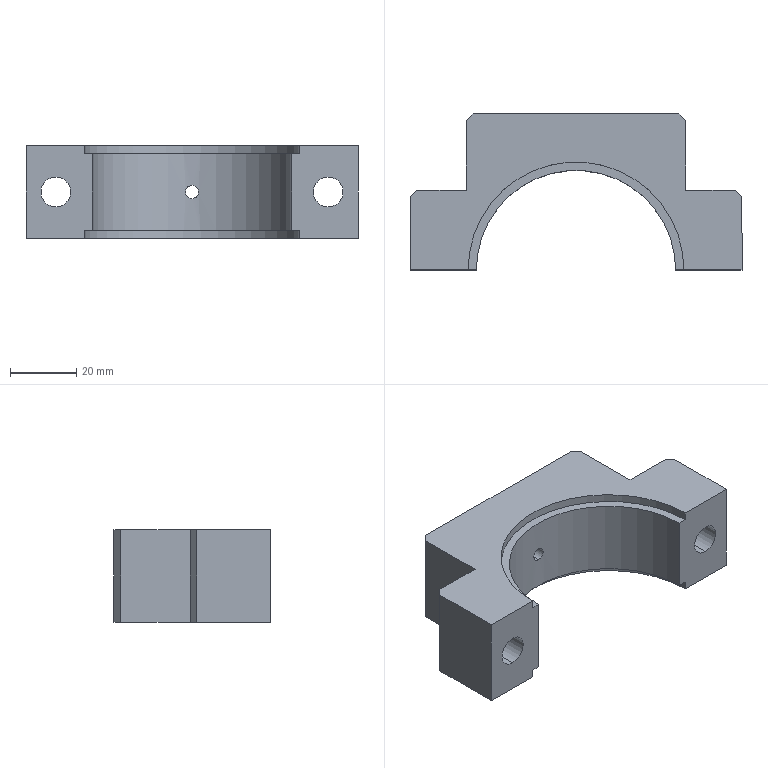Part | SolidWorks | features HoleWzd 3, ICE 2, Chamfer 1, Extrusion 1 | 1 solid | 30 faces | box 100 x 47 x 28 mm | volume 65054 mm3 | plane 17 | cylinder 11 | cone 2 | commonest cylinder face diameters 9 x4 4 x2 7 x2 65 x2 60 x1
STEP:
#1=CARTESIAN_POINT('',(0.,30.,12.));
#2=VERTEX_POINT('',#1);
#3=CARTESIAN_POINT('',(0.,30.,16.));
#4=VERTEX_POINT('',#3);
#5=CARTESIAN_POINT('',(0.,30.,12.));
#6=CARTESIAN_POINT('',(-0.261,30.,12.));
#7=CARTESIAN_POINT('',(-0.5242,29.996,12.052));
#8=CARTESIAN_POINT('',(-1.006,29.984,12.252));
#9=CARTESIAN_POINT('',(-1.229,29.975,12.401));
#10=CARTESIAN_POINT('',(-1.505,29.962,12.677));
#11=CARTESIAN_POINT('',(-1.59,29.958,12.78));
#12=CARTESIAN_POINT('',(-1.735,29.95,12.997));
#13=CARTESIAN_POINT('',(-1.797,29.946,13.112));
#14=CARTESIAN_POINT('',(-1.897,29.94,13.354));
#15=CARTESIAN_POINT('',(-1.936,29.937,13.481));
#16=CARTESIAN_POINT('',(-1.987,29.934,13.737));
#17=CARTESIAN_POINT('',(-2.,29.933,13.866));
#18=CARTESIAN_POINT('',(-2.,29.933,14.13));
#19=CARTESIAN_POINT('',(-1.987,29.934,14.261));
#20=CARTESIAN_POINT('',(-1.937,29.937,14.516));
#21=CARTESIAN_POINT('',(-1.898,29.94,14.643));
#22=CARTESIAN_POINT('',(-1.798,29.946,14.886));
#23=CARTESIAN_POINT('',(-1.737,29.95,15.001));
#24=CARTESIAN_POINT('',(-1.592,29.958,15.218));
#25=CARTESIAN_POINT('',(-1.507,29.962,15.321));
#26=CARTESIAN_POINT('',(-1.323,29.971,15.506));
#27=CARTESIAN_POINT('',(-1.222,29.975,15.588));
#28=CARTESIAN_POINT('',(-1.004,29.983,15.735));
#29=CARTESIAN_POINT('',(-0.8877,29.987,15.797));
#30=CARTESIAN_POINT('',(-0.5269,29.996,15.947));
#31=CARTESIAN_POINT('',(-0.2643,30.,16.));
#32=CARTESIAN_POINT('',(0.,30.,16.));
#33=B_SPLINE_CURVE_WITH_KNOTS('',3,(#5,#6,#7,#8,#9,#10,#11,#12,#13,#14,#15,#16,#17,#18,#19,#20,#21,#22,#23,#24,#25,#26,#27,#28,#29,#30,#31,#32),.UNSPECIFIED.,.F.,.F.,(4,2,2,2,2,2,2,2,2,2,2,2,2,4),(0.006255,0.007036,0.007818,0.008209,0.0086,0.00899,0.009381,0.009772,0.01016,0.01055,0.01094,0.01134,0.01173,0.01251),.UNSPECIFIED.);
#34=EDGE_CURVE('',#2,#4,#33,.T.);
#35=ORIENTED_EDGE('',*,*,#34,.F.);
#36=CARTESIAN_POINT('',(0.,33.099,12.));
#37=VERTEX_POINT('',#36);
#38=CARTESIAN_POINT('',(0.,47.,12.));
#39=DIRECTION('',(0.,1.,0.));
#40=VECTOR('',#39,1000.);
#41=LINE('',#38,#40);
#42=EDGE_CURVE('',#2,#37,#41,.T.);
#43=ORIENTED_EDGE('',*,*,#42,.T.);
#44=CARTESIAN_POINT('',(0.,33.099,16.));
#45=VERTEX_POINT('',#44);
#46=CARTESIAN_POINT('',(0.,33.099,14.));
#47=DIRECTION('',(0.,-1.,0.));
#48=DIRECTION('',(0.,0.,1.));
#49=AXIS2_PLACEMENT_3D('',#46,#47,#48);
#50=CIRCLE('',#49,2.);
#51=EDGE_CURVE('',#45,#37,#50,.T.);
#52=ORIENTED_EDGE('',*,*,#51,.F.);
#53=CARTESIAN_POINT('',(0.,47.,16.));
#54=DIRECTION('',(0.,1.,0.));
#55=VECTOR('',#54,1000.);
#56=LINE('',#53,#55);
#57=EDGE_CURVE('',#4,#45,#56,.T.);
#58=ORIENTED_EDGE('',*,*,#57,.F.);
#59=EDGE_LOOP('',(#35,#43,#52,#58));
#60=FACE_OUTER_BOUND('',#59,.T.);
#61=CARTESIAN_POINT('',(0.,47.,14.));
#62=DIRECTION('',(0.,1.,0.));
#63=DIRECTION('',(0.,0.,1.));
#64=AXIS2_PLACEMENT_3D('',#61,#62,#63);
#65=CYLINDRICAL_SURFACE('',#64,2.);
#66=ADVANCED_FACE('',(#60),#65,.F.);
#67=CARTESIAN_POINT('',(-41.,0.,9.5));
#68=VERTEX_POINT('',#67);
#69=CARTESIAN_POINT('',(-41.,0.,18.5));
#70=VERTEX_POINT('',#69);
#71=CARTESIAN_POINT('',(-41.,0.,14.));
#72=DIRECTION('',(0.,1.,0.));
#73=DIRECTION('',(0.,0.,1.));
#74=AXIS2_PLACEMENT_3D('',#71,#72,#73);
#75=CIRCLE('',#74,4.5);
#76=EDGE_CURVE('',#68,#70,#75,.T.);
#77=ORIENTED_EDGE('',*,*,#76,.F.);
#78=CARTESIAN_POINT('',(-41.,24.,9.5));
#79=VERTEX_POINT('',#78);
#80=CARTESIAN_POINT('',(-41.,24.,9.5));
#81=DIRECTION('',(0.,1.,0.));
#82=VECTOR('',#81,1000.);
#83=LINE('',#80,#82);
#84=EDGE_CURVE('',#68,#79,#83,.T.);
#85=ORIENTED_EDGE('',*,*,#84,.T.);
#86=CARTESIAN_POINT('',(-41.,24.,18.5));
#87=VERTEX_POINT('',#86);
#88=CARTESIAN_POINT('',(-41.,24.,14.));
#89=DIRECTION('',(0.,1.,0.));
#90=DIRECTION('',(0.,0.,1.));
#91=AXIS2_PLACEMENT_3D('',#88,#89,#90);
#92=CIRCLE('',#91,4.5);
#93=EDGE_CURVE('',#79,#87,#92,.T.);
#94=ORIENTED_EDGE('',*,*,#93,.T.);
#95=CARTESIAN_POINT('',(-41.,24.,18.5));
#96=DIRECTION('',(0.,1.,0.));
#97=VECTOR('',#96,1000.);
#98=LINE('',#95,#97);
#99=EDGE_CURVE('',#70,#87,#98,.T.);
#100=ORIENTED_EDGE('',*,*,#99,.F.);
#101=EDGE_LOOP('',(#77,#85,#94,#100));
#102=FACE_OUTER_BOUND('',#101,.T.);
#103=CARTESIAN_POINT('',(-41.,24.,14.));
#104=DIRECTION('',(0.,1.,0.));
#105=DIRECTION('',(0.,0.,1.));
#106=AXIS2_PLACEMENT_3D('',#103,#104,#105);
#107=CYLINDRICAL_SURFACE('',#106,4.5);
#108=ADVANCED_FACE('',(#102),#107,.F.);
#109=CARTESIAN_POINT('',(41.,0.,9.5));
#110=VERTEX_POINT('',#109);
#111=CARTESIAN_POINT('',(41.,0.,18.5));
#112=VERTEX_POINT('',#111);
#113=CARTESIAN_POINT('',(41.,0.,14.));
#114=DIRECTION('',(0.,1.,0.));
#115=DIRECTION('',(0.,0.,1.));
#116=AXIS2_PLACEMENT_3D('',#113,#114,#115);
#117=CIRCLE('',#116,4.5);
#118=EDGE_CURVE('',#110,#112,#117,.T.);
#119=ORIENTED_EDGE('',*,*,#118,.F.);
#120=CARTESIAN_POINT('',(41.,24.,9.5));
#121=VERTEX_POINT('',#120);
#122=CARTESIAN_POINT('',(41.,24.,9.5));
#123=DIRECTION('',(0.,1.,0.));
#124=VECTOR('',#123,1000.);
#125=LINE('',#122,#124);
#126=EDGE_CURVE('',#110,#121,#125,.T.);
#127=ORIENTED_EDGE('',*,*,#126,.T.);
#128=CARTESIAN_POINT('',(41.,24.,18.5));
#129=VERTEX_POINT('',#128);
#130=CARTESIAN_POINT('',(41.,24.,14.));
#131=DIRECTION('',(0.,1.,0.));
#132=DIRECTION('',(0.,0.,1.));
#133=AXIS2_PLACEMENT_3D('',#130,#131,#132);
#134=CIRCLE('',#133,4.5);
#135=EDGE_CURVE('',#121,#129,#134,.T.);
#136=ORIENTED_EDGE('',*,*,#135,.T.);
#137=CARTESIAN_POINT('',(41.,24.,18.5));
#138=DIRECTION('',(0.,1.,0.));
#139=VECTOR('',#138,1000.);
#140=LINE('',#137,#139);
#141=EDGE_CURVE('',#112,#129,#140,.T.);
#142=ORIENTED_EDGE('',*,*,#141,.F.);
#143=EDGE_LOOP('',(#119,#127,#136,#142));
#144=FACE_OUTER_BOUND('',#143,.T.);
#145=CARTESIAN_POINT('',(41.,24.,14.));
#146=DIRECTION('',(0.,1.,0.));
#147=DIRECTION('',(0.,0.,1.));
#148=AXIS2_PLACEMENT_3D('',#145,#146,#147);
#149=CYLINDRICAL_SURFACE('',#148,4.5);
#150=ADVANCED_FACE('',(#144),#149,.F.);
#151=CARTESIAN_POINT('',(0.,34.,10.5));
#152=VERTEX_POINT('',#151);
#153=CARTESIAN_POINT('',(0.,34.,17.5));
#154=VERTEX_POINT('',#153);
#155=CARTESIAN_POINT('',(0.,34.,14.));
#156=DIRECTION('',(0.,1.,0.));
#157=DIRECTION('',(0.,0.,1.));
#158=AXIS2_PLACEMENT_3D('',#155,#156,#157);
#159=CIRCLE('',#158,3.5);
#160=EDGE_CURVE('',#152,#154,#159,.T.);
#161=ORIENTED_EDGE('',*,*,#160,.F.);
#162=CARTESIAN_POINT('',(0.,47.,10.5));
#163=VERTEX_POINT('',#162);
#164=CARTESIAN_POINT('',(0.,47.,10.5));
#165=DIRECTION('',(0.,1.,0.));
#166=VECTOR('',#165,1000.);
#167=LINE('',#164,#166);
#168=EDGE_CURVE('',#152,#163,#167,.T.);
#169=ORIENTED_EDGE('',*,*,#168,.T.);
#170=CARTESIAN_POINT('',(0.,47.,17.5));
#171=VERTEX_POINT('',#170);
#172=CARTESIAN_POINT('',(0.,47.,14.));
#173=DIRECTION('',(0.,1.,0.));
#174=DIRECTION('',(0.,0.,1.));
#175=AXIS2_PLACEMENT_3D('',#172,#173,#174);
#176=CIRCLE('',#175,3.5);
#177=EDGE_CURVE('',#163,#171,#176,.T.);
#178=ORIENTED_EDGE('',*,*,#177,.T.);
#179=CARTESIAN_POINT('',(0.,47.,17.5));
#180=DIRECTION('',(0.,1.,0.));
#181=VECTOR('',#180,1000.);
#182=LINE('',#179,#181);
#183=EDGE_CURVE('',#154,#171,#182,.T.);
#184=ORIENTED_EDGE('',*,*,#183,.F.);
#185=EDGE_LOOP('',(#161,#169,#178,#184));
#186=FACE_OUTER_BOUND('',#185,.T.);
#187=CARTESIAN_POINT('',(0.,47.,14.));
#188=DIRECTION('',(0.,1.,0.));
#189=DIRECTION('',(0.,0.,1.));
#190=AXIS2_PLACEMENT_3D('',#187,#188,#189);
#191=CYLINDRICAL_SURFACE('',#190,3.5);
#192=ADVANCED_FACE('',(#186),#191,.F.);
#193=ORIENTED_EDGE('',*,*,#51,.T.);
#194=CARTESIAN_POINT('',(0.,34.,10.5));
#195=DIRECTION('',(0.,0.515,-0.8572));
#196=VECTOR('',#195,1000.);
#197=LINE('',#194,#196);
#198=EDGE_CURVE('',#37,#152,#197,.T.);
#199=ORIENTED_EDGE('',*,*,#198,.T.);
#200=ORIENTED_EDGE('',*,*,#160,.T.);
#201=CARTESIAN_POINT('',(0.,34.,17.5));
#202=DIRECTION('',(0.,0.515,0.8572));
#203=VECTOR('',#202,1000.);
#204=LINE('',#201,#203);
#205=EDGE_CURVE('',#45,#154,#204,.T.);
#206=ORIENTED_EDGE('',*,*,#205,.F.);
#207=EDGE_LOOP('',(#193,#199,#200,#206));
#208=FACE_OUTER_BOUND('',#207,.T.);
#209=CARTESIAN_POINT('',(0.,34.,14.));
#210=DIRECTION('',(0.,1.,0.));
#211=DIRECTION('',(0.,0.,1.));
#212=AXIS2_PLACEMENT_3D('',#209,#210,#211);
#213=CONICAL_SURFACE('',#212,3.5,1.03);
#214=ADVANCED_FACE('',(#208),#213,.F.);
#215=CARTESIAN_POINT('',(0.,30.,16.));
#216=CARTESIAN_POINT('',(0.1322,30.,16.));
#217=CARTESIAN_POINT('',(0.2622,29.999,15.987));
#218=CARTESIAN_POINT('',(0.5178,29.996,15.936));
#219=CARTESIAN_POINT('',(0.6449,29.993,15.898));
#220=CARTESIAN_POINT('',(0.8871,29.987,15.797));
#221=CARTESIAN_POINT('',(1.002,29.983,15.736));
#222=CARTESIAN_POINT('',(1.219,29.975,15.591));
#223=CARTESIAN_POINT('',(1.322,29.971,15.506));
#224=CARTESIAN_POINT('',(1.599,29.958,15.229));
#225=CARTESIAN_POINT('',(1.748,29.949,15.006));
#226=CARTESIAN_POINT('',(1.947,29.937,14.525));
#227=CARTESIAN_POINT('',(2.,29.933,14.262));
#228=CARTESIAN_POINT('',(2.,29.933,13.87));
#229=CARTESIAN_POINT('',(1.987,29.934,13.738));
#230=CARTESIAN_POINT('',(1.936,29.937,13.481));
#231=CARTESIAN_POINT('',(1.898,29.94,13.356));
#232=CARTESIAN_POINT('',(1.798,29.946,13.114));
#233=CARTESIAN_POINT('',(1.735,29.95,12.997));
#234=CARTESIAN_POINT('',(1.591,29.958,12.78));
#235=CARTESIAN_POINT('',(1.508,29.962,12.679));
#236=CARTESIAN_POINT('',(1.321,29.971,12.493));
#237=CARTESIAN_POINT('',(1.22,29.975,12.41));
#238=CARTESIAN_POINT('',(1.003,29.983,12.265));
#239=CARTESIAN_POINT('',(0.8865,29.987,12.202));
#240=CARTESIAN_POINT('',(0.6442,29.993,12.102));
#241=CARTESIAN_POINT('',(0.5195,29.996,12.064));
#242=CARTESIAN_POINT('',(0.2631,29.999,12.013));
#243=CARTESIAN_POINT('',(0.1305,30.,12.));
#244=CARTESIAN_POINT('',(0.,30.,12.));
#245=B_SPLINE_CURVE_WITH_KNOTS('',3,(#215,#216,#217,#218,#219,#220,#221,#222,#223,#224,#225,#226,#227,#228,#229,#230,#231,#232,#233,#234,#235,#236,#237,#238,#239,#240,#241,#242,#243,#244),.UNSPECIFIED.,.F.,.F.,(4,2,2,2,2,2,2,2,2,2,2,2,2,2,4),(0.,0.0003909,0.0007818,0.001173,0.001564,0.002345,0.003127,0.003518,0.003909,0.0043,0.004691,0.005082,0.005473,0.005864,0.006255),.UNSPECIFIED.);
#246=EDGE_CURVE('',#4,#2,#245,.T.);
#247=ORIENTED_EDGE('',*,*,#246,.T.);
#248=ORIENTED_EDGE('',*,*,#34,.T.);
#249=EDGE_LOOP('',(#247,#248));
#250=FACE_BOUND('',#249,.T.);
#251=CARTESIAN_POINT('',(-30.,0.,25.5));
#252=VERTEX_POINT('',#251);
#253=CARTESIAN_POINT('',(30.,0.,25.5));
#254=VERTEX_POINT('',#253);
#255=CARTESIAN_POINT('',(0.,0.,25.5));
#256=DIRECTION('',(0.,0.,-1.));
#257=DIRECTION('',(1.,0.,0.));
#258=AXIS2_PLACEMENT_3D('',#255,#256,#257);
#259=CIRCLE('',#258,30.);
#260=EDGE_CURVE('',#252,#254,#259,.T.);
#261=ORIENTED_EDGE('',*,*,#260,.F.);
#262=CARTESIAN_POINT('',(-30.,0.,2.5));
#263=VERTEX_POINT('',#262);
#264=CARTESIAN_POINT('',(-30.,0.,28.));
#265=DIRECTION('',(0.,0.,-1.));
#266=VECTOR('',#265,1000.);
#267=LINE('',#264,#266);
#268=EDGE_CURVE('',#252,#263,#267,.T.);
#269=ORIENTED_EDGE('',*,*,#268,.T.);
#270=CARTESIAN_POINT('',(30.,0.,2.5));
#271=VERTEX_POINT('',#270);
#272=CARTESIAN_POINT('',(0.,0.,2.5));
#273=DIRECTION('',(0.,0.,1.));
#274=DIRECTION('',(-1.,0.,0.));
#275=AXIS2_PLACEMENT_3D('',#272,#273,#274);
#276=CIRCLE('',#275,30.);
#277=EDGE_CURVE('',#271,#263,#276,.T.);
#278=ORIENTED_EDGE('',*,*,#277,.F.);
#279=CARTESIAN_POINT('',(30.,0.,28.));
#280=DIRECTION('',(0.,0.,-1.));
#281=VECTOR('',#280,1000.);
#282=LINE('',#279,#281);
#283=EDGE_CURVE('',#254,#271,#282,.T.);
#284=ORIENTED_EDGE('',*,*,#283,.F.);
#285=EDGE_LOOP('',(#261,#269,#278,#284));
#286=FACE_OUTER_BOUND('',#285,.T.);
#287=CARTESIAN_POINT('',(0.,0.,28.));
#288=DIRECTION('',(0.,0.,-1.));
#289=DIRECTION('',(-1.,0.,0.));
#290=AXIS2_PLACEMENT_3D('',#287,#288,#289);
#291=CYLINDRICAL_SURFACE('',#290,30.);
#292=ADVANCED_FACE('',(#250,#286),#291,.F.);
#293=CARTESIAN_POINT('',(-50.,22.,28.));
#294=VERTEX_POINT('',#293);
#295=CARTESIAN_POINT('',(-50.,0.,28.));
#296=VERTEX_POINT('',#295);
#297=CARTESIAN_POINT('',(-50.,0.,28.));
#298=DIRECTION('',(0.,-1.,0.));
#299=VECTOR('',#298,1000.);
#300=LINE('',#297,#299);
#301=EDGE_CURVE('',#294,#296,#300,.T.);
#302=ORIENTED_EDGE('',*,*,#301,.F.);
#303=CARTESIAN_POINT('',(-50.,22.,0.));
#304=VERTEX_POINT('',#303);
#305=CARTESIAN_POINT('',(-50.,22.,28.));
#306=DIRECTION('',(0.,0.,-1.));
#307=VECTOR('',#306,1000.);
#308=LINE('',#305,#307);
#309=EDGE_CURVE('',#294,#304,#308,.T.);
#310=ORIENTED_EDGE('',*,*,#309,.T.);
#311=CARTESIAN_POINT('',(-50.,0.,0.));
#312=VERTEX_POINT('',#311);
#313=CARTESIAN_POINT('',(-50.,0.,0.));
#314=DIRECTION('',(0.,-1.,0.));
#315=VECTOR('',#314,1000.);
#316=LINE('',#313,#315);
#317=EDGE_CURVE('',#304,#312,#316,.T.);
#318=ORIENTED_EDGE('',*,*,#317,.T.);
#319=CARTESIAN_POINT('',(-50.,0.,28.));
#320=DIRECTION('',(0.,0.,-1.));
#321=VECTOR('',#320,1000.);
#322=LINE('',#319,#321);
#323=EDGE_CURVE('',#296,#312,#322,.T.);
#324=ORIENTED_EDGE('',*,*,#323,.F.);
#325=EDGE_LOOP('',(#302,#310,#318,#324));
#326=FACE_OUTER_BOUND('',#325,.T.);
#327=CARTESIAN_POINT('',(-50.,0.,28.));
#328=DIRECTION('',(1.,0.,0.));
#329=DIRECTION('',(0.,0.,-1.));
#330=AXIS2_PLACEMENT_3D('',#327,#328,#329);
#331=PLANE('',#330);
#332=ADVANCED_FACE('',(#326),#331,.F.);
#333=CARTESIAN_POINT('',(-41.,0.,14.));
#334=DIRECTION('',(0.,1.,0.));
#335=DIRECTION('',(0.,0.,1.));
#336=AXIS2_PLACEMENT_3D('',#333,#334,#335);
#337=CIRCLE('',#336,4.5);
#338=EDGE_CURVE('',#70,#68,#337,.T.);
#339=ORIENTED_EDGE('',*,*,#338,.T.);
#340=ORIENTED_EDGE('',*,*,#76,.T.);
#341=EDGE_LOOP('',(#339,#340));
#342=FACE_BOUND('',#341,.T.);
#343=CARTESIAN_POINT('',(-32.5,0.,25.5));
#344=VERTEX_POINT('',#343);
#345=CARTESIAN_POINT('',(-50.,0.,25.5));
#346=DIRECTION('',(1.,0.,0.));
#347=VECTOR('',#346,1000.);
#348=LINE('',#345,#347);
#349=EDGE_CURVE('',#344,#252,#348,.T.);
#350=ORIENTED_EDGE('',*,*,#349,.F.);
#351=CARTESIAN_POINT('',(-32.5,0.,28.));
#352=VERTEX_POINT('',#351);
#353=CARTESIAN_POINT('',(-32.5,0.,25.5));
#354=DIRECTION('',(0.,0.,1.));
#355=VECTOR('',#354,1000.);
#356=LINE('',#353,#355);
#357=EDGE_CURVE('',#344,#352,#356,.T.);
#358=ORIENTED_EDGE('',*,*,#357,.T.);
#359=CARTESIAN_POINT('',(-50.,0.,28.));
#360=DIRECTION('',(1.,0.,0.));
#361=VECTOR('',#360,1000.);
#362=LINE('',#359,#361);
#363=EDGE_CURVE('',#296,#352,#362,.T.);
#364=ORIENTED_EDGE('',*,*,#363,.F.);
#365=ORIENTED_EDGE('',*,*,#323,.T.);
#366=CARTESIAN_POINT('',(-32.5,0.,0.));
#367=VERTEX_POINT('',#366);
#368=CARTESIAN_POINT('',(-50.,0.,0.));
#369=DIRECTION('',(1.,0.,0.));
#370=VECTOR('',#369,1000.);
#371=LINE('',#368,#370);
#372=EDGE_CURVE('',#312,#367,#371,.T.);
#373=ORIENTED_EDGE('',*,*,#372,.T.);
#374=CARTESIAN_POINT('',(-32.5,0.,2.5));
#375=VERTEX_POINT('',#374);
#376=CARTESIAN_POINT('',(-32.5,0.,2.5));
#377=DIRECTION('',(0.,0.,1.));
#378=VECTOR('',#377,1000.);
#379=LINE('',#376,#378);
#380=EDGE_CURVE('',#367,#375,#379,.T.);
#381=ORIENTED_EDGE('',*,*,#380,.T.);
#382=CARTESIAN_POINT('',(-50.,0.,2.5));
#383=DIRECTION('',(-1.,0.,0.));
#384=VECTOR('',#383,1000.);
#385=LINE('',#382,#384);
#386=EDGE_CURVE('',#263,#375,#385,.T.);
#387=ORIENTED_EDGE('',*,*,#386,.F.);
#388=ORIENTED_EDGE('',*,*,#268,.F.);
#389=EDGE_LOOP('',(#350,#358,#364,#365,#373,#381,#387,#388));
#390=FACE_OUTER_BOUND('',#389,.T.);
#391=CARTESIAN_POINT('',(-50.,0.,28.));
#392=DIRECTION('',(0.,1.,0.));
#393=DIRECTION('',(-1.,0.,0.));
#394=AXIS2_PLACEMENT_3D('',#391,#392,#393);
#395=PLANE('',#394);
#396=ADVANCED_FACE('',(#342,#390),#395,.F.);
#397=CARTESIAN_POINT('',(41.,0.,14.));
#398=DIRECTION('',(0.,1.,0.));
#399=DIRECTION('',(0.,0.,1.));
#400=AXIS2_PLACEMENT_3D('',#397,#398,#399);
#401=CIRCLE('',#400,4.5);
#402=EDGE_CURVE('',#112,#110,#401,.T.);
#403=ORIENTED_EDGE('',*,*,#402,.T.);
#404=ORIENTED_EDGE('',*,*,#118,.T.);
#405=EDGE_LOOP('',(#403,#404));
#406=FACE_BOUND('',#405,.T.);
#407=CARTESIAN_POINT('',(32.5,0.,28.));
#408=VERTEX_POINT('',#407);
#409=CARTESIAN_POINT('',(50.,0.,28.));
#410=VERTEX_POINT('',#409);
#411=CARTESIAN_POINT('',(30.,0.,28.));
#412=DIRECTION('',(1.,0.,0.));
#413=VECTOR('',#412,1000.);
#414=LINE('',#411,#413);
#415=EDGE_CURVE('',#408,#410,#414,.T.);
#416=ORIENTED_EDGE('',*,*,#415,.F.);
#417=CARTESIAN_POINT('',(32.5,0.,25.5));
#418=VERTEX_POINT('',#417);
#419=CARTESIAN_POINT('',(32.5,0.,25.5));
#420=DIRECTION('',(0.,0.,-1.));
#421=VECTOR('',#420,1000.);
#422=LINE('',#419,#421);
#423=EDGE_CURVE('',#408,#418,#422,.T.);
#424=ORIENTED_EDGE('',*,*,#423,.T.);
#425=CARTESIAN_POINT('',(30.,0.,25.5));
#426=DIRECTION('',(1.,0.,0.));
#427=VECTOR('',#426,1000.);
#428=LINE('',#425,#427);
#429=EDGE_CURVE('',#254,#418,#428,.T.);
#430=ORIENTED_EDGE('',*,*,#429,.F.);
#431=ORIENTED_EDGE('',*,*,#283,.T.);
#432=CARTESIAN_POINT('',(32.5,0.,2.5));
#433=VERTEX_POINT('',#432);
#434=CARTESIAN_POINT('',(30.,0.,2.5));
#435=DIRECTION('',(-1.,0.,0.));
#436=VECTOR('',#435,1000.);
#437=LINE('',#434,#436);
#438=EDGE_CURVE('',#433,#271,#437,.T.);
#439=ORIENTED_EDGE('',*,*,#438,.F.);
#440=CARTESIAN_POINT('',(32.5,0.,0.));
#441=VERTEX_POINT('',#440);
#442=CARTESIAN_POINT('',(32.5,0.,2.5));
#443=DIRECTION('',(0.,0.,-1.));
#444=VECTOR('',#443,1000.);
#445=LINE('',#442,#444);
#446=EDGE_CURVE('',#433,#441,#445,.T.);
#447=ORIENTED_EDGE('',*,*,#446,.T.);
#448=CARTESIAN_POINT('',(50.,0.,0.));
#449=VERTEX_POINT('',#448);
#450=CARTESIAN_POINT('',(30.,0.,0.));
#451=DIRECTION('',(1.,0.,0.));
#452=VECTOR('',#451,1000.);
#453=LINE('',#450,#452);
#454=EDGE_CURVE('',#441,#449,#453,.T.);
#455=ORIENTED_EDGE('',*,*,#454,.T.);
#456=CARTESIAN_POINT('',(50.,0.,28.));
#457=DIRECTION('',(0.,0.,-1.));
#458=VECTOR('',#457,1000.);
#459=LINE('',#456,#458);
#460=EDGE_CURVE('',#410,#449,#459,.T.);
#461=ORIENTED_EDGE('',*,*,#460,.F.);
#462=EDGE_LOOP('',(#416,#424,#430,#431,#439,#447,#455,#461));
#463=FACE_OUTER_BOUND('',#462,.T.);
#464=CARTESIAN_POINT('',(30.,0.,28.));
#465=DIRECTION('',(0.,1.,0.));
#466=DIRECTION('',(-1.,0.,0.));
#467=AXIS2_PLACEMENT_3D('',#464,#465,#466);
#468=PLANE('',#467);
#469=ADVANCED_FACE('',(#406,#463),#468,.F.);
#470=CARTESIAN_POINT('',(50.,22.,0.));
#471=VERTEX_POINT('',#470);
#472=CARTESIAN_POINT('',(50.,0.,0.));
#473=DIRECTION('',(0.,1.,0.));
#474=VECTOR('',#473,1000.);
#475=LINE('',#472,#474);
#476=EDGE_CURVE('',#449,#471,#475,.T.);
#477=ORIENTED_EDGE('',*,*,#476,.T.);
#478=CARTESIAN_POINT('',(50.,22.,28.));
#479=VERTEX_POINT('',#478);
#480=CARTESIAN_POINT('',(50.,22.,28.));
#481=DIRECTION('',(0.,0.,1.));
#482=VECTOR('',#481,1000.);
#483=LINE('',#480,#482);
#484=EDGE_CURVE('',#471,#479,#483,.T.);
#485=ORIENTED_EDGE('',*,*,#484,.T.);
#486=CARTESIAN_POINT('',(50.,0.,28.));
#487=DIRECTION('',(0.,1.,0.));
#488=VECTOR('',#487,1000.);
#489=LINE('',#486,#488);
#490=EDGE_CURVE('',#410,#479,#489,.T.);
#491=ORIENTED_EDGE('',*,*,#490,.F.);
#492=ORIENTED_EDGE('',*,*,#460,.T.);
#493=EDGE_LOOP('',(#477,#485,#491,#492));
#494=FACE_OUTER_BOUND('',#493,.T.);
#495=CARTESIAN_POINT('',(50.,0.,28.));
#496=DIRECTION('',(-1.,0.,0.));
#497=DIRECTION('',(0.,-1.,0.));
#498=AXIS2_PLACEMENT_3D('',#495,#496,#497);
#499=PLANE('',#498);
#500=ADVANCED_FACE('',(#494),#499,.F.);
#501=CARTESIAN_POINT('',(41.,24.,14.));
#502=DIRECTION('',(0.,1.,0.));
#503=DIRECTION('',(0.,0.,1.));
#504=AXIS2_PLACEMENT_3D('',#501,#502,#503);
#505=CIRCLE('',#504,4.5);
#506=EDGE_CURVE('',#129,#121,#505,.T.);
#507=ORIENTED_EDGE('',*,*,#506,.F.);
#508=ORIENTED_EDGE('',*,*,#135,.F.);
#509=EDGE_LOOP('',(#507,#508));
#510=FACE_BOUND('',#509,.T.);
#511=CARTESIAN_POINT('',(48.,24.,28.));
#512=VERTEX_POINT('',#511);
#513=CARTESIAN_POINT('',(33.,24.,28.));
#514=VERTEX_POINT('',#513);
#515=CARTESIAN_POINT('',(50.,24.,28.));
#516=DIRECTION('',(-1.,0.,0.));
#517=VECTOR('',#516,1000.);
#518=LINE('',#515,#517);
#519=EDGE_CURVE('',#512,#514,#518,.T.);
#520=ORIENTED_EDGE('',*,*,#519,.F.);
#521=CARTESIAN_POINT('',(48.,24.,0.));
#522=VERTEX_POINT('',#521);
#523=CARTESIAN_POINT('',(48.,24.,28.));
#524=DIRECTION('',(0.,0.,-1.));
#525=VECTOR('',#524,1000.);
#526=LINE('',#523,#525);
#527=EDGE_CURVE('',#512,#522,#526,.T.);
#528=ORIENTED_EDGE('',*,*,#527,.T.);
#529=CARTESIAN_POINT('',(33.,24.,0.));
#530=VERTEX_POINT('',#529);
#531=CARTESIAN_POINT('',(50.,24.,0.));
#532=DIRECTION('',(-1.,0.,0.));
#533=VECTOR('',#532,1000.);
#534=LINE('',#531,#533);
#535=EDGE_CURVE('',#522,#530,#534,.T.);
#536=ORIENTED_EDGE('',*,*,#535,.T.);
#537=CARTESIAN_POINT('',(33.,24.,28.));
#538=DIRECTION('',(0.,0.,-1.));
#539=VECTOR('',#538,1000.);
#540=LINE('',#537,#539);
#541=EDGE_CURVE('',#514,#530,#540,.T.);
#542=ORIENTED_EDGE('',*,*,#541,.F.);
#543=EDGE_LOOP('',(#520,#528,#536,#542));
#544=FACE_OUTER_BOUND('',#543,.T.);
#545=CARTESIAN_POINT('',(50.,24.,28.));
#546=DIRECTION('',(0.,-1.,0.));
#547=DIRECTION('',(1.,0.,0.));
#548=AXIS2_PLACEMENT_3D('',#545,#546,#547);
#549=PLANE('',#548);
#550=ADVANCED_FACE('',(#510,#544),#549,.F.);
#551=CARTESIAN_POINT('',(33.,45.,0.));
#552=VERTEX_POINT('',#551);
#553=CARTESIAN_POINT('',(33.,24.,0.));
#554=DIRECTION('',(0.,1.,0.));
#555=VECTOR('',#554,1000.);
#556=LINE('',#553,#555);
#557=EDGE_CURVE('',#530,#552,#556,.T.);
#558=ORIENTED_EDGE('',*,*,#557,.T.);
#559=CARTESIAN_POINT('',(33.,45.,28.));
#560=VERTEX_POINT('',#559);
#561=CARTESIAN_POINT('',(33.,45.,28.));
#562=DIRECTION('',(0.,0.,1.));
#563=VECTOR('',#562,1000.);
#564=LINE('',#561,#563);
#565=EDGE_CURVE('',#552,#560,#564,.T.);
#566=ORIENTED_EDGE('',*,*,#565,.T.);
#567=CARTESIAN_POINT('',(33.,24.,28.));
#568=DIRECTION('',(0.,1.,0.));
#569=VECTOR('',#568,1000.);
#570=LINE('',#567,#569);
#571=EDGE_CURVE('',#514,#560,#570,.T.);
#572=ORIENTED_EDGE('',*,*,#571,.F.);
#573=ORIENTED_EDGE('',*,*,#541,.T.);
#574=EDGE_LOOP('',(#558,#566,#572,#573));
#575=FACE_OUTER_BOUND('',#574,.T.);
#576=CARTESIAN_POINT('',(33.,24.,28.));
#577=DIRECTION('',(-1.,0.,0.));
#578=DIRECTION('',(0.,-1.,0.));
#579=AXIS2_PLACEMENT_3D('',#576,#577,#578);
#580=PLANE('',#579);
#581=ADVANCED_FACE('',(#575),#580,.F.);
#582=CARTESIAN_POINT('',(0.,47.,14.));
#583=DIRECTION('',(0.,1.,0.));
#584=DIRECTION('',(0.,0.,1.));
#585=AXIS2_PLACEMENT_3D('',#582,#583,#584);
#586=CIRCLE('',#585,3.5);
#587=EDGE_CURVE('',#171,#163,#586,.T.);
#588=ORIENTED_EDGE('',*,*,#587,.F.);
#589=ORIENTED_EDGE('',*,*,#177,.F.);
#590=EDGE_LOOP('',(#588,#589));
#591=FACE_BOUND('',#590,.T.);
#592=CARTESIAN_POINT('',(31.,47.,28.));
#593=VERTEX_POINT('',#592);
#594=CARTESIAN_POINT('',(-31.,47.,28.));
#595=VERTEX_POINT('',#594);
#596=CARTESIAN_POINT('',(-33.,47.,28.));
#597=DIRECTION('',(-1.,0.,0.));
#598=VECTOR('',#597,1000.);
#599=LINE('',#596,#598);
#600=EDGE_CURVE('',#593,#595,#599,.T.);
#601=ORIENTED_EDGE('',*,*,#600,.F.);
#602=CARTESIAN_POINT('',(31.,47.,0.));
#603=VERTEX_POINT('',#602);
#604=CARTESIAN_POINT('',(31.,47.,28.));
#605=DIRECTION('',(0.,0.,-1.));
#606=VECTOR('',#605,1000.);
#607=LINE('',#604,#606);
#608=EDGE_CURVE('',#593,#603,#607,.T.);
#609=ORIENTED_EDGE('',*,*,#608,.T.);
#610=CARTESIAN_POINT('',(-31.,47.,0.));
#611=VERTEX_POINT('',#610);
#612=CARTESIAN_POINT('',(-33.,47.,0.));
#613=DIRECTION('',(-1.,0.,0.));
#614=VECTOR('',#613,1000.);
#615=LINE('',#612,#614);
#616=EDGE_CURVE('',#603,#611,#615,.T.);
#617=ORIENTED_EDGE('',*,*,#616,.T.);
#618=CARTESIAN_POINT('',(-31.,47.,28.));
#619=DIRECTION('',(0.,0.,1.));
#620=VECTOR('',#619,1000.);
#621=LINE('',#618,#620);
#622=EDGE_CURVE('',#611,#595,#621,.T.);
#623=ORIENTED_EDGE('',*,*,#622,.T.);
#624=EDGE_LOOP('',(#601,#609,#617,#623));
#625=FACE_OUTER_BOUND('',#624,.T.);
#626=CARTESIAN_POINT('',(-33.,47.,28.));
#627=DIRECTION('',(0.,-1.,0.));
#628=DIRECTION('',(1.,0.,0.));
#629=AXIS2_PLACEMENT_3D('',#626,#627,#628);
#630=PLANE('',#629);
#631=ADVANCED_FACE('',(#591,#625),#630,.F.);
#632=CARTESIAN_POINT('',(-33.,45.,28.));
#633=VERTEX_POINT('',#632);
#634=CARTESIAN_POINT('',(-33.,24.,28.));
#635=VERTEX_POINT('',#634);
#636=CARTESIAN_POINT('',(-33.,24.,28.));
#637=DIRECTION('',(0.,-1.,0.));
#638=VECTOR('',#637,1000.);
#639=LINE('',#636,#638);
#640=EDGE_CURVE('',#633,#635,#639,.T.);
#641=ORIENTED_EDGE('',*,*,#640,.F.);
#642=CARTESIAN_POINT('',(-33.,45.,0.));
#643=VERTEX_POINT('',#642);
#644=CARTESIAN_POINT('',(-33.,45.,28.));
#645=DIRECTION('',(0.,0.,-1.));
#646=VECTOR('',#645,1000.);
#647=LINE('',#644,#646);
#648=EDGE_CURVE('',#633,#643,#647,.T.);
#649=ORIENTED_EDGE('',*,*,#648,.T.);
#650=CARTESIAN_POINT('',(-33.,24.,0.));
#651=VERTEX_POINT('',#650);
#652=CARTESIAN_POINT('',(-33.,24.,0.));
#653=DIRECTION('',(0.,-1.,0.));
#654=VECTOR('',#653,1000.);
#655=LINE('',#652,#654);
#656=EDGE_CURVE('',#643,#651,#655,.T.);
#657=ORIENTED_EDGE('',*,*,#656,.T.);
#658=CARTESIAN_POINT('',(-33.,24.,28.));
#659=DIRECTION('',(0.,0.,-1.));
#660=VECTOR('',#659,1000.);
#661=LINE('',#658,#660);
#662=EDGE_CURVE('',#635,#651,#661,.T.);
#663=ORIENTED_EDGE('',*,*,#662,.F.);
#664=EDGE_LOOP('',(#641,#649,#657,#663));
#665=FACE_OUTER_BOUND('',#664,.T.);
#666=CARTESIAN_POINT('',(-33.,24.,28.));
#667=DIRECTION('',(1.,0.,0.));
#668=DIRECTION('',(0.,1.,0.));
#669=AXIS2_PLACEMENT_3D('',#666,#667,#668);
#670=PLANE('',#669);
#671=ADVANCED_FACE('',(#665),#670,.F.);
#672=CARTESIAN_POINT('',(-41.,24.,14.));
#673=DIRECTION('',(0.,1.,0.));
#674=DIRECTION('',(0.,0.,1.));
#675=AXIS2_PLACEMENT_3D('',#672,#673,#674);
#676=CIRCLE('',#675,4.5);
#677=EDGE_CURVE('',#87,#79,#676,.T.);
#678=ORIENTED_EDGE('',*,*,#677,.F.);
#679=ORIENTED_EDGE('',*,*,#93,.F.);
#680=EDGE_LOOP('',(#678,#679));
#681=FACE_BOUND('',#680,.T.);
#682=CARTESIAN_POINT('',(-48.,24.,0.));
#683=VERTEX_POINT('',#682);
#684=CARTESIAN_POINT('',(-50.,24.,0.));
#685=DIRECTION('',(-1.,0.,0.));
#686=VECTOR('',#685,1000.);
#687=LINE('',#684,#686);
#688=EDGE_CURVE('',#651,#683,#687,.T.);
#689=ORIENTED_EDGE('',*,*,#688,.T.);
#690=CARTESIAN_POINT('',(-48.,24.,28.));
#691=VERTEX_POINT('',#690);
#692=CARTESIAN_POINT('',(-48.,24.,28.));
#693=DIRECTION('',(0.,0.,1.));
#694=VECTOR('',#693,1000.);
#695=LINE('',#692,#694);
#696=EDGE_CURVE('',#683,#691,#695,.T.);
#697=ORIENTED_EDGE('',*,*,#696,.T.);
#698=CARTESIAN_POINT('',(-50.,24.,28.));
#699=DIRECTION('',(-1.,0.,0.));
#700=VECTOR('',#699,1000.);
#701=LINE('',#698,#700);
#702=EDGE_CURVE('',#635,#691,#701,.T.);
#703=ORIENTED_EDGE('',*,*,#702,.F.);
#704=ORIENTED_EDGE('',*,*,#662,.T.);
#705=EDGE_LOOP('',(#689,#697,#703,#704));
#706=FACE_OUTER_BOUND('',#705,.T.);
#707=CARTESIAN_POINT('',(-50.,24.,28.));
#708=DIRECTION('',(0.,-1.,0.));
#709=DIRECTION('',(1.,0.,0.));
#710=AXIS2_PLACEMENT_3D('',#707,#708,#709);
#711=PLANE('',#710);
#712=ADVANCED_FACE('',(#681,#706),#711,.F.);
#713=CARTESIAN_POINT('',(0.,0.,28.));
#714=DIRECTION('',(0.,0.,1.));
#715=DIRECTION('',(1.,0.,0.));
#716=AXIS2_PLACEMENT_3D('',#713,#714,#715);
#717=CIRCLE('',#716,32.5);
#718=EDGE_CURVE('',#408,#352,#717,.T.);
#719=ORIENTED_EDGE('',*,*,#718,.F.);
#720=ORIENTED_EDGE('',*,*,#415,.T.);
#721=ORIENTED_EDGE('',*,*,#490,.T.);
#722=CARTESIAN_POINT('',(36.,36.,28.));
#723=DIRECTION('',(-0.7071,0.7071,0.));
#724=VECTOR('',#723,1000.);
#725=LINE('',#722,#724);
#726=EDGE_CURVE('',#479,#512,#725,.T.);
#727=ORIENTED_EDGE('',*,*,#726,.T.);
#728=ORIENTED_EDGE('',*,*,#519,.T.);
#729=ORIENTED_EDGE('',*,*,#571,.T.);
#730=CARTESIAN_POINT('',(39.,39.,28.));
#731=DIRECTION('',(-0.7071,0.7071,0.));
#732=VECTOR('',#731,1000.);
#733=LINE('',#730,#732);
#734=EDGE_CURVE('',#560,#593,#733,.T.);
#735=ORIENTED_EDGE('',*,*,#734,.T.);
#736=ORIENTED_EDGE('',*,*,#600,.T.);
#737=CARTESIAN_POINT('',(-39.,39.,28.));
#738=DIRECTION('',(-0.7071,-0.7071,0.));
#739=VECTOR('',#738,1000.);
#740=LINE('',#737,#739);
#741=EDGE_CURVE('',#595,#633,#740,.T.);
#742=ORIENTED_EDGE('',*,*,#741,.T.);
#743=ORIENTED_EDGE('',*,*,#640,.T.);
#744=ORIENTED_EDGE('',*,*,#702,.T.);
#745=CARTESIAN_POINT('',(-36.,36.,28.));
#746=DIRECTION('',(-0.7071,-0.7071,0.));
#747=VECTOR('',#746,1000.);
#748=LINE('',#745,#747);
#749=EDGE_CURVE('',#691,#294,#748,.T.);
#750=ORIENTED_EDGE('',*,*,#749,.T.);
#751=ORIENTED_EDGE('',*,*,#301,.T.);
#752=ORIENTED_EDGE('',*,*,#363,.T.);
#753=EDGE_LOOP('',(#719,#720,#721,#727,#728,#729,#735,#736,#742,#743,#744,#750,#751,#752));
#754=FACE_OUTER_BOUND('',#753,.T.);
#755=CARTESIAN_POINT('',(0.,0.,28.));
#756=DIRECTION('',(0.,0.,1.));
#757=DIRECTION('',(1.,0.,0.));
#758=AXIS2_PLACEMENT_3D('',#755,#756,#757);
#759=PLANE('',#758);
#760=ADVANCED_FACE('',(#754),#759,.T.);
#761=ORIENTED_EDGE('',*,*,#454,.F.);
#762=CARTESIAN_POINT('',(0.,0.,0.));
#763=DIRECTION('',(0.,0.,-1.));
#764=DIRECTION('',(-1.,0.,0.));
#765=AXIS2_PLACEMENT_3D('',#762,#763,#764);
#766=CIRCLE('',#765,32.5);
#767=EDGE_CURVE('',#367,#441,#766,.T.);
#768=ORIENTED_EDGE('',*,*,#767,.F.);
#769=ORIENTED_EDGE('',*,*,#372,.F.);
#770=ORIENTED_EDGE('',*,*,#317,.F.);
#771=CARTESIAN_POINT('',(-50.,22.,0.));
#772=DIRECTION('',(0.7071,0.7071,0.));
#773=VECTOR('',#772,1000.);
#774=LINE('',#771,#773);
#775=EDGE_CURVE('',#304,#683,#774,.T.);
#776=ORIENTED_EDGE('',*,*,#775,.T.);
#777=ORIENTED_EDGE('',*,*,#688,.F.);
#778=ORIENTED_EDGE('',*,*,#656,.F.);
#779=CARTESIAN_POINT('',(-33.,45.,0.));
#780=DIRECTION('',(0.7071,0.7071,0.));
#781=VECTOR('',#780,1000.);
#782=LINE('',#779,#781);
#783=EDGE_CURVE('',#643,#611,#782,.T.);
#784=ORIENTED_EDGE('',*,*,#783,.T.);
#785=ORIENTED_EDGE('',*,*,#616,.F.);
#786=CARTESIAN_POINT('',(31.,47.,0.));
#787=DIRECTION('',(0.7071,-0.7071,0.));
#788=VECTOR('',#787,1000.);
#789=LINE('',#786,#788);
#790=EDGE_CURVE('',#603,#552,#789,.T.);
#791=ORIENTED_EDGE('',*,*,#790,.T.);
#792=ORIENTED_EDGE('',*,*,#557,.F.);
#793=ORIENTED_EDGE('',*,*,#535,.F.);
#794=CARTESIAN_POINT('',(48.,24.,0.));
#795=DIRECTION('',(0.7071,-0.7071,0.));
#796=VECTOR('',#795,1000.);
#797=LINE('',#794,#796);
#798=EDGE_CURVE('',#522,#471,#797,.T.);
#799=ORIENTED_EDGE('',*,*,#798,.T.);
#800=ORIENTED_EDGE('',*,*,#476,.F.);
#801=EDGE_LOOP('',(#761,#768,#769,#770,#776,#777,#778,#784,#785,#791,#792,#793,#799,#800));
#802=FACE_OUTER_BOUND('',#801,.T.);
#803=CARTESIAN_POINT('',(0.,0.,0.));
#804=DIRECTION('',(0.,0.,1.));
#805=DIRECTION('',(1.,0.,0.));
#806=AXIS2_PLACEMENT_3D('',#803,#804,#805);
#807=PLANE('',#806);
#808=ADVANCED_FACE('',(#802),#807,.F.);
#809=ORIENTED_EDGE('',*,*,#726,.F.);
#810=ORIENTED_EDGE('',*,*,#484,.F.);
#811=ORIENTED_EDGE('',*,*,#798,.F.);
#812=ORIENTED_EDGE('',*,*,#527,.F.);
#813=EDGE_LOOP('',(#809,#810,#811,#812));
#814=FACE_OUTER_BOUND('',#813,.T.);
#815=CARTESIAN_POINT('',(48.,24.,28.));
#816=DIRECTION('',(-0.7071,-0.7071,0.));
#817=DIRECTION('',(0.,0.,-1.));
#818=AXIS2_PLACEMENT_3D('',#815,#816,#817);
#819=PLANE('',#818);
#820=ADVANCED_FACE('',(#814),#819,.F.);
#821=ORIENTED_EDGE('',*,*,#734,.F.);
#822=ORIENTED_EDGE('',*,*,#565,.F.);
#823=ORIENTED_EDGE('',*,*,#790,.F.);
#824=ORIENTED_EDGE('',*,*,#608,.F.);
#825=EDGE_LOOP('',(#821,#822,#823,#824));
#826=FACE_OUTER_BOUND('',#825,.T.);
#827=CARTESIAN_POINT('',(31.,47.,28.));
#828=DIRECTION('',(-0.7071,-0.7071,0.));
#829=DIRECTION('',(0.,0.,-1.));
#830=AXIS2_PLACEMENT_3D('',#827,#828,#829);
#831=PLANE('',#830);
#832=ADVANCED_FACE('',(#826),#831,.F.);
#833=ORIENTED_EDGE('',*,*,#741,.F.);
#834=ORIENTED_EDGE('',*,*,#622,.F.);
#835=ORIENTED_EDGE('',*,*,#783,.F.);
#836=ORIENTED_EDGE('',*,*,#648,.F.);
#837=EDGE_LOOP('',(#833,#834,#835,#836));
#838=FACE_OUTER_BOUND('',#837,.T.);
#839=CARTESIAN_POINT('',(-33.,45.,28.));
#840=DIRECTION('',(0.7071,-0.7071,0.));
#841=DIRECTION('',(0.,0.,-1.));
#842=AXIS2_PLACEMENT_3D('',#839,#840,#841);
#843=PLANE('',#842);
#844=ADVANCED_FACE('',(#838),#843,.F.);
#845=ORIENTED_EDGE('',*,*,#749,.F.);
#846=ORIENTED_EDGE('',*,*,#696,.F.);
#847=ORIENTED_EDGE('',*,*,#775,.F.);
#848=ORIENTED_EDGE('',*,*,#309,.F.);
#849=EDGE_LOOP('',(#845,#846,#847,#848));
#850=FACE_OUTER_BOUND('',#849,.T.);
#851=CARTESIAN_POINT('',(-50.,22.,28.));
#852=DIRECTION('',(0.7071,-0.7071,0.));
#853=DIRECTION('',(0.,0.,-1.));
#854=AXIS2_PLACEMENT_3D('',#851,#852,#853);
#855=PLANE('',#854);
#856=ADVANCED_FACE('',(#850),#855,.F.);
#857=ORIENTED_EDGE('',*,*,#198,.F.);
#858=CARTESIAN_POINT('',(0.,33.099,14.));
#859=DIRECTION('',(0.,-1.,0.));
#860=DIRECTION('',(0.,0.,1.));
#861=AXIS2_PLACEMENT_3D('',#858,#859,#860);
#862=CIRCLE('',#861,2.);
#863=EDGE_CURVE('',#37,#45,#862,.T.);
#864=ORIENTED_EDGE('',*,*,#863,.T.);
#865=ORIENTED_EDGE('',*,*,#205,.T.);
#866=CARTESIAN_POINT('',(0.,34.,14.));
#867=DIRECTION('',(0.,1.,0.));
#868=DIRECTION('',(0.,0.,1.));
#869=AXIS2_PLACEMENT_3D('',#866,#867,#868);
#870=CIRCLE('',#869,3.5);
#871=EDGE_CURVE('',#154,#152,#870,.T.);
#872=ORIENTED_EDGE('',*,*,#871,.T.);
#873=EDGE_LOOP('',(#857,#864,#865,#872));
#874=FACE_OUTER_BOUND('',#873,.T.);
#875=CARTESIAN_POINT('',(0.,34.,14.));
#876=DIRECTION('',(0.,1.,0.));
#877=DIRECTION('',(0.,0.,1.));
#878=AXIS2_PLACEMENT_3D('',#875,#876,#877);
#879=CONICAL_SURFACE('',#878,3.5,1.03);
#880=ADVANCED_FACE('',(#874),#879,.F.);
#881=ORIENTED_EDGE('',*,*,#168,.F.);
#882=ORIENTED_EDGE('',*,*,#871,.F.);
#883=ORIENTED_EDGE('',*,*,#183,.T.);
#884=ORIENTED_EDGE('',*,*,#587,.T.);
#885=EDGE_LOOP('',(#881,#882,#883,#884));
#886=FACE_OUTER_BOUND('',#885,.T.);
#887=CARTESIAN_POINT('',(0.,47.,14.));
#888=DIRECTION('',(0.,1.,0.));
#889=DIRECTION('',(0.,0.,1.));
#890=AXIS2_PLACEMENT_3D('',#887,#888,#889);
#891=CYLINDRICAL_SURFACE('',#890,3.5);
#892=ADVANCED_FACE('',(#886),#891,.F.);
#893=ORIENTED_EDGE('',*,*,#126,.F.);
#894=ORIENTED_EDGE('',*,*,#402,.F.);
#895=ORIENTED_EDGE('',*,*,#141,.T.);
#896=ORIENTED_EDGE('',*,*,#506,.T.);
#897=EDGE_LOOP('',(#893,#894,#895,#896));
#898=FACE_OUTER_BOUND('',#897,.T.);
#899=CARTESIAN_POINT('',(41.,24.,14.));
#900=DIRECTION('',(0.,1.,0.));
#901=DIRECTION('',(0.,0.,1.));
#902=AXIS2_PLACEMENT_3D('',#899,#900,#901);
#903=CYLINDRICAL_SURFACE('',#902,4.5);
#904=ADVANCED_FACE('',(#898),#903,.F.);
#905=ORIENTED_EDGE('',*,*,#84,.F.);
#906=ORIENTED_EDGE('',*,*,#338,.F.);
#907=ORIENTED_EDGE('',*,*,#99,.T.);
#908=ORIENTED_EDGE('',*,*,#677,.T.);
#909=EDGE_LOOP('',(#905,#906,#907,#908));
#910=FACE_OUTER_BOUND('',#909,.T.);
#911=CARTESIAN_POINT('',(-41.,24.,14.));
#912=DIRECTION('',(0.,1.,0.));
#913=DIRECTION('',(0.,0.,1.));
#914=AXIS2_PLACEMENT_3D('',#911,#912,#913);
#915=CYLINDRICAL_SURFACE('',#914,4.5);
#916=ADVANCED_FACE('',(#910),#915,.F.);
#917=ORIENTED_EDGE('',*,*,#386,.T.);
#918=CARTESIAN_POINT('',(0.,0.,2.5));
#919=DIRECTION('',(0.,0.,-1.));
#920=DIRECTION('',(-1.,0.,0.));
#921=AXIS2_PLACEMENT_3D('',#918,#919,#920);
#922=CIRCLE('',#921,32.5);
#923=EDGE_CURVE('',#375,#433,#922,.T.);
#924=ORIENTED_EDGE('',*,*,#923,.T.);
#925=ORIENTED_EDGE('',*,*,#438,.T.);
#926=ORIENTED_EDGE('',*,*,#277,.T.);
#927=EDGE_LOOP('',(#917,#924,#925,#926));
#928=FACE_OUTER_BOUND('',#927,.T.);
#929=CARTESIAN_POINT('',(0.,0.,2.5));
#930=DIRECTION('',(0.,0.,-1.));
#931=DIRECTION('',(-1.,0.,0.));
#932=AXIS2_PLACEMENT_3D('',#929,#930,#931);
#933=PLANE('',#932);
#934=ADVANCED_FACE('',(#928),#933,.T.);
#935=ORIENTED_EDGE('',*,*,#767,.T.);
#936=ORIENTED_EDGE('',*,*,#446,.F.);
#937=ORIENTED_EDGE('',*,*,#923,.F.);
#938=ORIENTED_EDGE('',*,*,#380,.F.);
#939=EDGE_LOOP('',(#935,#936,#937,#938));
#940=FACE_OUTER_BOUND('',#939,.T.);
#941=CARTESIAN_POINT('',(0.,0.,2.5));
#942=DIRECTION('',(0.,0.,-1.));
#943=DIRECTION('',(-1.,0.,0.));
#944=AXIS2_PLACEMENT_3D('',#941,#942,#943);
#945=CYLINDRICAL_SURFACE('',#944,32.5);
#946=ADVANCED_FACE('',(#940),#945,.F.);
#947=ORIENTED_EDGE('',*,*,#349,.T.);
#948=ORIENTED_EDGE('',*,*,#260,.T.);
#949=ORIENTED_EDGE('',*,*,#429,.T.);
#950=CARTESIAN_POINT('',(0.,0.,25.5));
#951=DIRECTION('',(0.,0.,1.));
#952=DIRECTION('',(1.,0.,0.));
#953=AXIS2_PLACEMENT_3D('',#950,#951,#952);
#954=CIRCLE('',#953,32.5);
#955=EDGE_CURVE('',#418,#344,#954,.T.);
#956=ORIENTED_EDGE('',*,*,#955,.T.);
#957=EDGE_LOOP('',(#947,#948,#949,#956));
#958=FACE_OUTER_BOUND('',#957,.T.);
#959=CARTESIAN_POINT('',(0.,0.,25.5));
#960=DIRECTION('',(0.,0.,1.));
#961=DIRECTION('',(1.,0.,0.));
#962=AXIS2_PLACEMENT_3D('',#959,#960,#961);
#963=PLANE('',#962);
#964=ADVANCED_FACE('',(#958),#963,.T.);
#965=ORIENTED_EDGE('',*,*,#955,.F.);
#966=ORIENTED_EDGE('',*,*,#423,.F.);
#967=ORIENTED_EDGE('',*,*,#718,.T.);
#968=ORIENTED_EDGE('',*,*,#357,.F.);
#969=EDGE_LOOP('',(#965,#966,#967,#968));
#970=FACE_OUTER_BOUND('',#969,.T.);
#971=CARTESIAN_POINT('',(0.,0.,25.5));
#972=DIRECTION('',(0.,0.,1.));
#973=DIRECTION('',(1.,0.,0.));
#974=AXIS2_PLACEMENT_3D('',#971,#972,#973);
#975=CYLINDRICAL_SURFACE('',#974,32.5);
#976=ADVANCED_FACE('',(#970),#975,.F.);
#977=ORIENTED_EDGE('',*,*,#42,.F.);
#978=ORIENTED_EDGE('',*,*,#246,.F.);
#979=ORIENTED_EDGE('',*,*,#57,.T.);
#980=ORIENTED_EDGE('',*,*,#863,.F.);
#981=EDGE_LOOP('',(#977,#978,#979,#980));
#982=FACE_OUTER_BOUND('',#981,.T.);
#983=CARTESIAN_POINT('',(0.,47.,14.));
#984=DIRECTION('',(0.,1.,0.));
#985=DIRECTION('',(0.,0.,1.));
#986=AXIS2_PLACEMENT_3D('',#983,#984,#985);
#987=CYLINDRICAL_SURFACE('',#986,2.);
#988=ADVANCED_FACE('',(#982),#987,.F.);
#989=CLOSED_SHELL('',(#66,#108,#150,#192,#214,#292,#332,#396,#469,#500,#550,#581,#631,#671,#712,#760,#808,#820,#832,#844,#856,#880,#892,#904,#916,#934,#946,#964,#976,#988));
#990=MANIFOLD_SOLID_BREP('',#989);
#991=CARTESIAN_POINT('',(0.,0.,0.));
#992=DIRECTION('',(0.,0.,1.));
#993=DIRECTION('',(1.,0.,0.));
#994=AXIS2_PLACEMENT_3D('',#991,#992,#993);
#995=(LENGTH_UNIT()NAMED_UNIT(*)SI_UNIT(.MILLI.,.METRE.));
#996=UNCERTAINTY_MEASURE_WITH_UNIT(LENGTH_MEASURE(0.00001),#995,'','');
#997=(NAMED_UNIT(*)PLANE_ANGLE_UNIT()SI_UNIT($,.RADIAN.));
#998=(NAMED_UNIT(*)SI_UNIT($,.STERADIAN.)SOLID_ANGLE_UNIT());
#999=(GEOMETRIC_REPRESENTATION_CONTEXT(3)GLOBAL_UNCERTAINTY_ASSIGNED_CONTEXT((#996))GLOBAL_UNIT_ASSIGNED_CONTEXT((#995,#997,#998))REPRESENTATION_CONTEXT('',''));
#1000=ADVANCED_BREP_SHAPE_REPRESENTATION('',(#990,#994),#999);